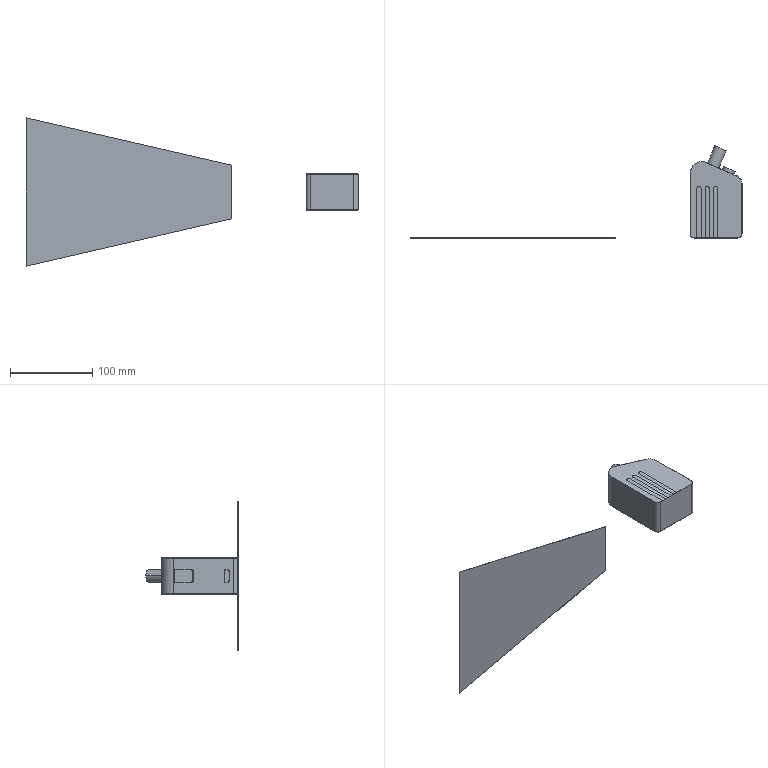Part | STEP file | ZLDS202_250 | 2 solids | 391 faces | box 403 x 111.961 x 180 mm | volume 243934 mm3 | cylinder 296 | plane 67 | spline 12 | cone 8 | torus 8 | commonest cylinder face diameters 4.2 x256 0.4 x10 3 x8 4 x8 5.22 x6 15 x4